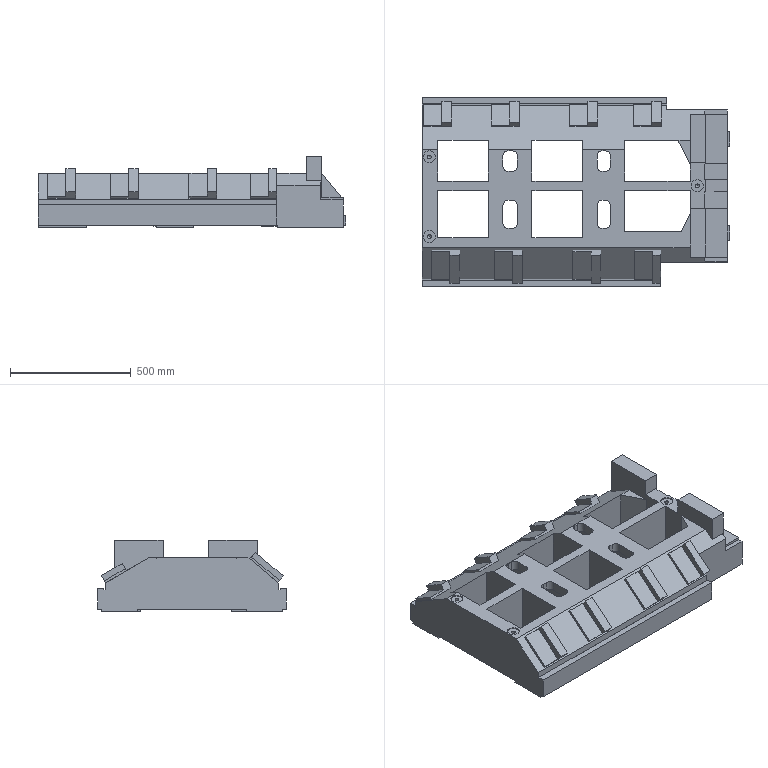Part | NX | features solid 2 | 1 solid | 255 faces | box 1275 x 780 x 295 mm | volume 102511793 mm3 | plane 228 | cylinder 22 | cone 3 | spline 2 | commonest cylinder face diameters 40 x16 16 x3 50 x3